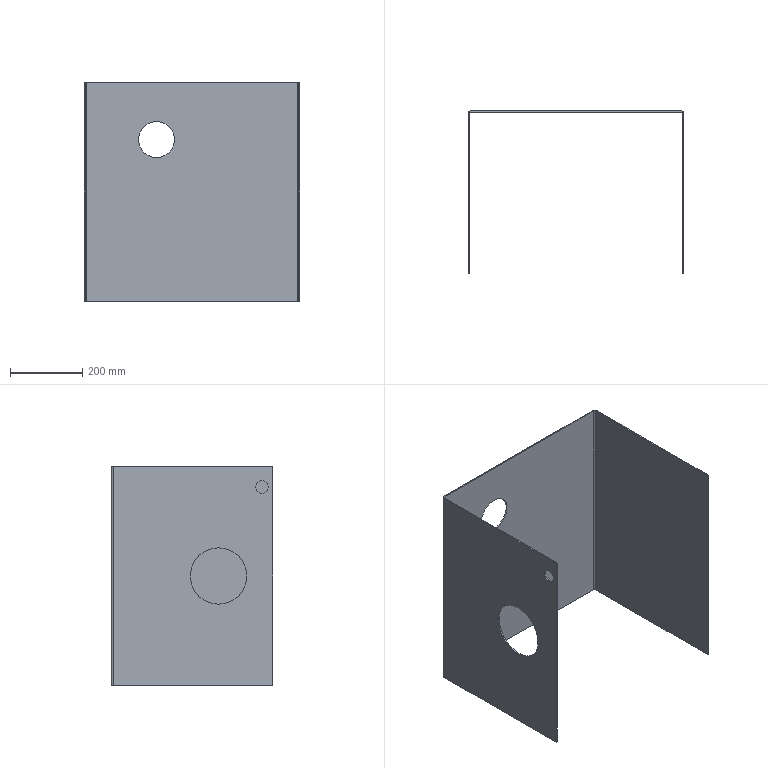Part | SolidWorks | features ICE 3, FlatPattern 1, SMBaseFlange 1, SheetMetal 1 | 1 solid | 32 faces | box 596 x 447 x 606 mm | volume 2607078 mm3 | plane 18 | cylinder 14 | commonest cylinder face diameters 6 x6 12 x2 35 x2 100 x2 156 x2
STEP:
#1=CARTESIAN_POINT('',(200.,447.,398.));
#2=VERTEX_POINT('',#1);
#3=CARTESIAN_POINT('',(200.,447.,498.));
#4=VERTEX_POINT('',#3);
#5=CARTESIAN_POINT('',(200.,447.,448.));
#6=DIRECTION('',(0.,1.,0.));
#7=DIRECTION('',(0.,0.,1.));
#8=AXIS2_PLACEMENT_3D('',#5,#6,#7);
#9=CIRCLE('',#8,50.);
#10=EDGE_CURVE('',#2,#4,#9,.T.);
#11=ORIENTED_EDGE('',*,*,#10,.T.);
#12=CARTESIAN_POINT('',(200.,444.,498.));
#13=VERTEX_POINT('',#12);
#14=CARTESIAN_POINT('',(200.,454.,498.));
#15=DIRECTION('',(0.,-1.,0.));
#16=VECTOR('',#15,1000.);
#17=LINE('',#14,#16);
#18=EDGE_CURVE('',#4,#13,#17,.T.);
#19=ORIENTED_EDGE('',*,*,#18,.T.);
#20=CARTESIAN_POINT('',(200.,444.,398.));
#21=VERTEX_POINT('',#20);
#22=CARTESIAN_POINT('',(200.,444.,448.));
#23=DIRECTION('',(0.,-1.,0.));
#24=DIRECTION('',(0.,0.,-1.));
#25=AXIS2_PLACEMENT_3D('',#22,#23,#24);
#26=CIRCLE('',#25,50.);
#27=EDGE_CURVE('',#13,#21,#26,.T.);
#28=ORIENTED_EDGE('',*,*,#27,.T.);
#29=CARTESIAN_POINT('',(200.,454.,398.));
#30=DIRECTION('',(0.,-1.,0.));
#31=VECTOR('',#30,1000.);
#32=LINE('',#29,#31);
#33=EDGE_CURVE('',#2,#21,#32,.T.);
#34=ORIENTED_EDGE('',*,*,#33,.F.);
#35=EDGE_LOOP('',(#11,#19,#28,#34));
#36=FACE_OUTER_BOUND('',#35,.T.);
#37=CARTESIAN_POINT('',(200.,454.,448.));
#38=DIRECTION('',(0.,-1.,0.));
#39=DIRECTION('',(0.,0.,-1.));
#40=AXIS2_PLACEMENT_3D('',#37,#38,#39);
#41=CYLINDRICAL_SURFACE('',#40,50.);
#42=ADVANCED_FACE('',(#36),#41,.F.);
#43=CARTESIAN_POINT('',(3.,30.,531.5));
#44=VERTEX_POINT('',#43);
#45=CARTESIAN_POINT('',(3.,30.,566.5));
#46=VERTEX_POINT('',#45);
#47=CARTESIAN_POINT('',(3.,30.,549.));
#48=DIRECTION('',(-1.,0.,0.));
#49=DIRECTION('',(0.,0.,1.));
#50=AXIS2_PLACEMENT_3D('',#47,#48,#49);
#51=CIRCLE('',#50,17.5);
#52=EDGE_CURVE('',#44,#46,#51,.T.);
#53=ORIENTED_EDGE('',*,*,#52,.F.);
#54=CARTESIAN_POINT('',(0.,30.,531.5));
#55=VERTEX_POINT('',#54);
#56=CARTESIAN_POINT('',(10.,30.,531.5));
#57=DIRECTION('',(-1.,0.,0.));
#58=VECTOR('',#57,1000.);
#59=LINE('',#56,#58);
#60=EDGE_CURVE('',#44,#55,#59,.T.);
#61=ORIENTED_EDGE('',*,*,#60,.T.);
#62=CARTESIAN_POINT('',(0.,30.,566.5));
#63=VERTEX_POINT('',#62);
#64=CARTESIAN_POINT('',(0.,30.,549.));
#65=DIRECTION('',(-1.,0.,0.));
#66=DIRECTION('',(0.,0.,1.));
#67=AXIS2_PLACEMENT_3D('',#64,#65,#66);
#68=CIRCLE('',#67,17.5);
#69=EDGE_CURVE('',#55,#63,#68,.T.);
#70=ORIENTED_EDGE('',*,*,#69,.T.);
#71=CARTESIAN_POINT('',(10.,30.,566.5));
#72=DIRECTION('',(-1.,0.,0.));
#73=VECTOR('',#72,1000.);
#74=LINE('',#71,#73);
#75=EDGE_CURVE('',#46,#63,#74,.T.);
#76=ORIENTED_EDGE('',*,*,#75,.F.);
#77=EDGE_LOOP('',(#53,#61,#70,#76));
#78=FACE_OUTER_BOUND('',#77,.T.);
#79=CARTESIAN_POINT('',(10.,30.,549.));
#80=DIRECTION('',(-1.,0.,0.));
#81=DIRECTION('',(0.,0.,1.));
#82=AXIS2_PLACEMENT_3D('',#79,#80,#81);
#83=CYLINDRICAL_SURFACE('',#82,17.5);
#84=ADVANCED_FACE('',(#78),#83,.F.);
#85=CARTESIAN_POINT('',(3.,150.,225.));
#86=VERTEX_POINT('',#85);
#87=CARTESIAN_POINT('',(3.,150.,381.));
#88=VERTEX_POINT('',#87);
#89=CARTESIAN_POINT('',(3.,150.,303.));
#90=DIRECTION('',(-1.,0.,0.));
#91=DIRECTION('',(0.,0.,1.));
#92=AXIS2_PLACEMENT_3D('',#89,#90,#91);
#93=CIRCLE('',#92,78.);
#94=EDGE_CURVE('',#86,#88,#93,.T.);
#95=ORIENTED_EDGE('',*,*,#94,.F.);
#96=CARTESIAN_POINT('',(0.,150.,225.));
#97=VERTEX_POINT('',#96);
#98=CARTESIAN_POINT('',(10.,150.,225.));
#99=DIRECTION('',(-1.,0.,0.));
#100=VECTOR('',#99,1000.);
#101=LINE('',#98,#100);
#102=EDGE_CURVE('',#86,#97,#101,.T.);
#103=ORIENTED_EDGE('',*,*,#102,.T.);
#104=CARTESIAN_POINT('',(0.,150.,381.));
#105=VERTEX_POINT('',#104);
#106=CARTESIAN_POINT('',(0.,150.,303.));
#107=DIRECTION('',(-1.,0.,0.));
#108=DIRECTION('',(0.,0.,1.));
#109=AXIS2_PLACEMENT_3D('',#106,#107,#108);
#110=CIRCLE('',#109,78.);
#111=EDGE_CURVE('',#97,#105,#110,.T.);
#112=ORIENTED_EDGE('',*,*,#111,.T.);
#113=CARTESIAN_POINT('',(10.,150.,381.));
#114=DIRECTION('',(-1.,0.,0.));
#115=VECTOR('',#114,1000.);
#116=LINE('',#113,#115);
#117=EDGE_CURVE('',#88,#105,#116,.T.);
#118=ORIENTED_EDGE('',*,*,#117,.F.);
#119=EDGE_LOOP('',(#95,#103,#112,#118));
#120=FACE_OUTER_BOUND('',#119,.T.);
#121=CARTESIAN_POINT('',(10.,150.,303.));
#122=DIRECTION('',(-1.,0.,0.));
#123=DIRECTION('',(0.,0.,1.));
#124=AXIS2_PLACEMENT_3D('',#121,#122,#123);
#125=CYLINDRICAL_SURFACE('',#124,78.);
#126=ADVANCED_FACE('',(#120),#125,.F.);
#127=CARTESIAN_POINT('',(593.,3.,606.));
#128=VERTEX_POINT('',#127);
#129=CARTESIAN_POINT('',(593.,0.,603.));
#130=VERTEX_POINT('',#129);
#131=CARTESIAN_POINT('',(593.,3.,603.));
#132=DIRECTION('',(1.,0.,0.));
#133=DIRECTION('',(0.,1.,0.));
#134=AXIS2_PLACEMENT_3D('',#131,#132,#133);
#135=CIRCLE('',#134,3.);
#136=EDGE_CURVE('',#128,#130,#135,.T.);
#137=ORIENTED_EDGE('',*,*,#136,.F.);
#138=CARTESIAN_POINT('',(593.,441.,606.));
#139=VERTEX_POINT('',#138);
#140=CARTESIAN_POINT('',(593.,447.,606.));
#141=DIRECTION('',(0.,-1.,0.));
#142=VECTOR('',#141,1000.);
#143=LINE('',#140,#142);
#144=EDGE_CURVE('',#139,#128,#143,.T.);
#145=ORIENTED_EDGE('',*,*,#144,.F.);
#146=CARTESIAN_POINT('',(593.,441.,0.));
#147=VERTEX_POINT('',#146);
#148=CARTESIAN_POINT('',(593.,441.,606.));
#149=DIRECTION('',(0.,0.,-1.));
#150=VECTOR('',#149,1000.);
#151=LINE('',#148,#150);
#152=EDGE_CURVE('',#139,#147,#151,.T.);
#153=ORIENTED_EDGE('',*,*,#152,.T.);
#154=CARTESIAN_POINT('',(593.,3.,0.));
#155=VERTEX_POINT('',#154);
#156=CARTESIAN_POINT('',(593.,447.,0.));
#157=DIRECTION('',(0.,-1.,0.));
#158=VECTOR('',#157,1000.);
#159=LINE('',#156,#158);
#160=EDGE_CURVE('',#147,#155,#159,.T.);
#161=ORIENTED_EDGE('',*,*,#160,.T.);
#162=CARTESIAN_POINT('',(593.,0.,3.));
#163=VERTEX_POINT('',#162);
#164=CARTESIAN_POINT('',(593.,3.,3.));
#165=DIRECTION('',(-1.,0.,0.));
#166=DIRECTION('',(0.,1.,0.));
#167=AXIS2_PLACEMENT_3D('',#164,#165,#166);
#168=CIRCLE('',#167,3.);
#169=EDGE_CURVE('',#155,#163,#168,.T.);
#170=ORIENTED_EDGE('',*,*,#169,.T.);
#171=CARTESIAN_POINT('',(593.,0.,606.));
#172=DIRECTION('',(0.,0.,-1.));
#173=VECTOR('',#172,1000.);
#174=LINE('',#171,#173);
#175=EDGE_CURVE('',#130,#163,#174,.T.);
#176=ORIENTED_EDGE('',*,*,#175,.F.);
#177=EDGE_LOOP('',(#137,#145,#153,#161,#170,#176));
#178=FACE_OUTER_BOUND('',#177,.T.);
#179=CARTESIAN_POINT('',(593.,447.,606.));
#180=DIRECTION('',(1.,0.,0.));
#181=DIRECTION('',(0.,1.,0.));
#182=AXIS2_PLACEMENT_3D('',#179,#180,#181);
#183=PLANE('',#182);
#184=ADVANCED_FACE('',(#178),#183,.F.);
#185=CARTESIAN_POINT('',(596.,441.,606.));
#186=VERTEX_POINT('',#185);
#187=CARTESIAN_POINT('',(596.,3.,606.));
#188=VERTEX_POINT('',#187);
#189=CARTESIAN_POINT('',(596.,447.,606.));
#190=DIRECTION('',(0.,-1.,0.));
#191=VECTOR('',#190,1000.);
#192=LINE('',#189,#191);
#193=EDGE_CURVE('',#186,#188,#192,.T.);
#194=ORIENTED_EDGE('',*,*,#193,.T.);
#195=CARTESIAN_POINT('',(596.,0.,603.));
#196=VERTEX_POINT('',#195);
#197=CARTESIAN_POINT('',(596.,3.,603.));
#198=DIRECTION('',(1.,0.,0.));
#199=DIRECTION('',(0.,1.,0.));
#200=AXIS2_PLACEMENT_3D('',#197,#198,#199);
#201=CIRCLE('',#200,3.);
#202=EDGE_CURVE('',#188,#196,#201,.T.);
#203=ORIENTED_EDGE('',*,*,#202,.T.);
#204=CARTESIAN_POINT('',(596.,0.,3.));
#205=VERTEX_POINT('',#204);
#206=CARTESIAN_POINT('',(596.,0.,606.));
#207=DIRECTION('',(0.,0.,-1.));
#208=VECTOR('',#207,1000.);
#209=LINE('',#206,#208);
#210=EDGE_CURVE('',#196,#205,#209,.T.);
#211=ORIENTED_EDGE('',*,*,#210,.T.);
#212=CARTESIAN_POINT('',(596.,3.,0.));
#213=VERTEX_POINT('',#212);
#214=CARTESIAN_POINT('',(596.,3.,3.));
#215=DIRECTION('',(-1.,0.,0.));
#216=DIRECTION('',(0.,1.,0.));
#217=AXIS2_PLACEMENT_3D('',#214,#215,#216);
#218=CIRCLE('',#217,3.);
#219=EDGE_CURVE('',#213,#205,#218,.T.);
#220=ORIENTED_EDGE('',*,*,#219,.F.);
#221=CARTESIAN_POINT('',(596.,441.,0.));
#222=VERTEX_POINT('',#221);
#223=CARTESIAN_POINT('',(596.,447.,0.));
#224=DIRECTION('',(0.,-1.,0.));
#225=VECTOR('',#224,1000.);
#226=LINE('',#223,#225);
#227=EDGE_CURVE('',#222,#213,#226,.T.);
#228=ORIENTED_EDGE('',*,*,#227,.F.);
#229=CARTESIAN_POINT('',(596.,441.,606.));
#230=DIRECTION('',(0.,0.,-1.));
#231=VECTOR('',#230,1000.);
#232=LINE('',#229,#231);
#233=EDGE_CURVE('',#186,#222,#232,.T.);
#234=ORIENTED_EDGE('',*,*,#233,.F.);
#235=EDGE_LOOP('',(#194,#203,#211,#220,#228,#234));
#236=FACE_OUTER_BOUND('',#235,.T.);
#237=CARTESIAN_POINT('',(596.,447.,606.));
#238=DIRECTION('',(1.,0.,0.));
#239=DIRECTION('',(0.,1.,0.));
#240=AXIS2_PLACEMENT_3D('',#237,#238,#239);
#241=PLANE('',#240);
#242=ADVANCED_FACE('',(#236),#241,.T.);
#243=ORIENTED_EDGE('',*,*,#144,.T.);
#244=CARTESIAN_POINT('',(593.,3.,606.));
#245=DIRECTION('',(1.,0.,0.));
#246=VECTOR('',#245,1000.);
#247=LINE('',#244,#246);
#248=EDGE_CURVE('',#128,#188,#247,.T.);
#249=ORIENTED_EDGE('',*,*,#248,.T.);
#250=ORIENTED_EDGE('',*,*,#193,.F.);
#251=CARTESIAN_POINT('',(596.,441.,606.));
#252=DIRECTION('',(-1.,0.,0.));
#253=VECTOR('',#252,1000.);
#254=LINE('',#251,#253);
#255=EDGE_CURVE('',#186,#139,#254,.T.);
#256=ORIENTED_EDGE('',*,*,#255,.T.);
#257=EDGE_LOOP('',(#243,#249,#250,#256));
#258=FACE_OUTER_BOUND('',#257,.T.);
#259=CARTESIAN_POINT('',(590.,444.,606.));
#260=DIRECTION('',(0.,0.,1.));
#261=DIRECTION('',(1.,0.,0.));
#262=AXIS2_PLACEMENT_3D('',#259,#260,#261);
#263=PLANE('',#262);
#264=ADVANCED_FACE('',(#258),#263,.T.);
#265=CARTESIAN_POINT('',(593.,0.,603.));
#266=DIRECTION('',(1.,0.,0.));
#267=VECTOR('',#266,1000.);
#268=LINE('',#265,#267);
#269=EDGE_CURVE('',#130,#196,#268,.T.);
#270=ORIENTED_EDGE('',*,*,#269,.F.);
#271=ORIENTED_EDGE('',*,*,#175,.T.);
#272=CARTESIAN_POINT('',(593.,0.,3.));
#273=DIRECTION('',(1.,0.,0.));
#274=VECTOR('',#273,1000.);
#275=LINE('',#272,#274);
#276=EDGE_CURVE('',#163,#205,#275,.T.);
#277=ORIENTED_EDGE('',*,*,#276,.T.);
#278=ORIENTED_EDGE('',*,*,#210,.F.);
#279=EDGE_LOOP('',(#270,#271,#277,#278));
#280=FACE_OUTER_BOUND('',#279,.T.);
#281=CARTESIAN_POINT('',(596.,0.,606.));
#282=DIRECTION('',(0.,-1.,0.));
#283=DIRECTION('',(0.,0.,-1.));
#284=AXIS2_PLACEMENT_3D('',#281,#282,#283);
#285=PLANE('',#284);
#286=ADVANCED_FACE('',(#280),#285,.T.);
#287=CARTESIAN_POINT('',(593.,3.,0.));
#288=DIRECTION('',(1.,0.,0.));
#289=VECTOR('',#288,1000.);
#290=LINE('',#287,#289);
#291=EDGE_CURVE('',#155,#213,#290,.T.);
#292=ORIENTED_EDGE('',*,*,#291,.F.);
#293=ORIENTED_EDGE('',*,*,#160,.F.);
#294=CARTESIAN_POINT('',(593.,441.,0.));
#295=DIRECTION('',(1.,0.,0.));
#296=VECTOR('',#295,1000.);
#297=LINE('',#294,#296);
#298=EDGE_CURVE('',#147,#222,#297,.T.);
#299=ORIENTED_EDGE('',*,*,#298,.T.);
#300=ORIENTED_EDGE('',*,*,#227,.T.);
#301=EDGE_LOOP('',(#292,#293,#299,#300));
#302=FACE_OUTER_BOUND('',#301,.T.);
#303=CARTESIAN_POINT('',(590.,441.,0.));
#304=DIRECTION('',(0.,0.,1.));
#305=DIRECTION('',(1.,0.,0.));
#306=AXIS2_PLACEMENT_3D('',#303,#304,#305);
#307=PLANE('',#306);
#308=ADVANCED_FACE('',(#302),#307,.F.);
#309=CARTESIAN_POINT('',(0.,30.,549.));
#310=DIRECTION('',(-1.,0.,0.));
#311=DIRECTION('',(0.,0.,1.));
#312=AXIS2_PLACEMENT_3D('',#309,#310,#311);
#313=CIRCLE('',#312,17.5);
#314=EDGE_CURVE('',#63,#55,#313,.T.);
#315=ORIENTED_EDGE('',*,*,#314,.F.);
#316=ORIENTED_EDGE('',*,*,#69,.F.);
#317=EDGE_LOOP('',(#315,#316));
#318=FACE_BOUND('',#317,.T.);
#319=CARTESIAN_POINT('',(0.,150.,303.));
#320=DIRECTION('',(-1.,0.,0.));
#321=DIRECTION('',(0.,0.,1.));
#322=AXIS2_PLACEMENT_3D('',#319,#320,#321);
#323=CIRCLE('',#322,78.);
#324=EDGE_CURVE('',#105,#97,#323,.T.);
#325=ORIENTED_EDGE('',*,*,#324,.F.);
#326=ORIENTED_EDGE('',*,*,#111,.F.);
#327=EDGE_LOOP('',(#325,#326));
#328=FACE_BOUND('',#327,.T.);
#329=CARTESIAN_POINT('',(0.,0.,603.));
#330=VERTEX_POINT('',#329);
#331=CARTESIAN_POINT('',(0.,0.,3.));
#332=VERTEX_POINT('',#331);
#333=CARTESIAN_POINT('',(0.,0.,606.));
#334=DIRECTION('',(0.,0.,-1.));
#335=VECTOR('',#334,1000.);
#336=LINE('',#333,#335);
#337=EDGE_CURVE('',#330,#332,#336,.T.);
#338=ORIENTED_EDGE('',*,*,#337,.F.);
#339=CARTESIAN_POINT('',(0.,3.,606.));
#340=VERTEX_POINT('',#339);
#341=CARTESIAN_POINT('',(0.,3.,603.));
#342=DIRECTION('',(-1.,0.,0.));
#343=DIRECTION('',(0.,0.,1.));
#344=AXIS2_PLACEMENT_3D('',#341,#342,#343);
#345=CIRCLE('',#344,3.);
#346=EDGE_CURVE('',#330,#340,#345,.T.);
#347=ORIENTED_EDGE('',*,*,#346,.T.);
#348=CARTESIAN_POINT('',(0.,441.,606.));
#349=VERTEX_POINT('',#348);
#350=CARTESIAN_POINT('',(0.,0.,606.));
#351=DIRECTION('',(0.,1.,0.));
#352=VECTOR('',#351,1000.);
#353=LINE('',#350,#352);
#354=EDGE_CURVE('',#340,#349,#353,.T.);
#355=ORIENTED_EDGE('',*,*,#354,.T.);
#356=CARTESIAN_POINT('',(0.,441.,0.));
#357=VERTEX_POINT('',#356);
#358=CARTESIAN_POINT('',(0.,441.,606.));
#359=DIRECTION('',(0.,0.,-1.));
#360=VECTOR('',#359,1000.);
#361=LINE('',#358,#360);
#362=EDGE_CURVE('',#349,#357,#361,.T.);
#363=ORIENTED_EDGE('',*,*,#362,.T.);
#364=CARTESIAN_POINT('',(0.,3.,0.));
#365=VERTEX_POINT('',#364);
#366=CARTESIAN_POINT('',(0.,0.,0.));
#367=DIRECTION('',(0.,1.,0.));
#368=VECTOR('',#367,1000.);
#369=LINE('',#366,#368);
#370=EDGE_CURVE('',#365,#357,#369,.T.);
#371=ORIENTED_EDGE('',*,*,#370,.F.);
#372=CARTESIAN_POINT('',(0.,3.,3.));
#373=DIRECTION('',(1.,0.,0.));
#374=DIRECTION('',(0.,0.,1.));
#375=AXIS2_PLACEMENT_3D('',#372,#373,#374);
#376=CIRCLE('',#375,3.);
#377=EDGE_CURVE('',#332,#365,#376,.T.);
#378=ORIENTED_EDGE('',*,*,#377,.F.);
#379=EDGE_LOOP('',(#338,#347,#355,#363,#371,#378));
#380=FACE_OUTER_BOUND('',#379,.T.);
#381=CARTESIAN_POINT('',(0.,0.,606.));
#382=DIRECTION('',(-1.,0.,0.));
#383=DIRECTION('',(0.,0.,1.));
#384=AXIS2_PLACEMENT_3D('',#381,#382,#383);
#385=PLANE('',#384);
#386=ADVANCED_FACE('',(#318,#328,#380),#385,.T.);
#387=CARTESIAN_POINT('',(3.,30.,549.));
#388=DIRECTION('',(-1.,0.,0.));
#389=DIRECTION('',(0.,0.,1.));
#390=AXIS2_PLACEMENT_3D('',#387,#388,#389);
#391=CIRCLE('',#390,17.5);
#392=EDGE_CURVE('',#46,#44,#391,.T.);
#393=ORIENTED_EDGE('',*,*,#392,.T.);
#394=ORIENTED_EDGE('',*,*,#52,.T.);
#395=EDGE_LOOP('',(#393,#394));
#396=FACE_BOUND('',#395,.T.);
#397=CARTESIAN_POINT('',(3.,150.,303.));
#398=DIRECTION('',(-1.,0.,0.));
#399=DIRECTION('',(0.,0.,1.));
#400=AXIS2_PLACEMENT_3D('',#397,#398,#399);
#401=CIRCLE('',#400,78.);
#402=EDGE_CURVE('',#88,#86,#401,.T.);
#403=ORIENTED_EDGE('',*,*,#402,.T.);
#404=ORIENTED_EDGE('',*,*,#94,.T.);
#405=EDGE_LOOP('',(#403,#404));
#406=FACE_BOUND('',#405,.T.);
#407=CARTESIAN_POINT('',(3.,0.,603.));
#408=VERTEX_POINT('',#407);
#409=CARTESIAN_POINT('',(3.,3.,606.));
#410=VERTEX_POINT('',#409);
#411=CARTESIAN_POINT('',(3.,3.,603.));
#412=DIRECTION('',(-1.,0.,0.));
#413=DIRECTION('',(0.,0.,1.));
#414=AXIS2_PLACEMENT_3D('',#411,#412,#413);
#415=CIRCLE('',#414,3.);
#416=EDGE_CURVE('',#408,#410,#415,.T.);
#417=ORIENTED_EDGE('',*,*,#416,.F.);
#418=CARTESIAN_POINT('',(3.,0.,3.));
#419=VERTEX_POINT('',#418);
#420=CARTESIAN_POINT('',(3.,0.,606.));
#421=DIRECTION('',(0.,0.,-1.));
#422=VECTOR('',#421,1000.);
#423=LINE('',#420,#422);
#424=EDGE_CURVE('',#408,#419,#423,.T.);
#425=ORIENTED_EDGE('',*,*,#424,.T.);
#426=CARTESIAN_POINT('',(3.,3.,0.));
#427=VERTEX_POINT('',#426);
#428=CARTESIAN_POINT('',(3.,3.,3.));
#429=DIRECTION('',(1.,0.,0.));
#430=DIRECTION('',(0.,0.,1.));
#431=AXIS2_PLACEMENT_3D('',#428,#429,#430);
#432=CIRCLE('',#431,3.);
#433=EDGE_CURVE('',#419,#427,#432,.T.);
#434=ORIENTED_EDGE('',*,*,#433,.T.);
#435=CARTESIAN_POINT('',(3.,441.,0.));
#436=VERTEX_POINT('',#435);
#437=CARTESIAN_POINT('',(3.,0.,0.));
#438=DIRECTION('',(0.,1.,0.));
#439=VECTOR('',#438,1000.);
#440=LINE('',#437,#439);
#441=EDGE_CURVE('',#427,#436,#440,.T.);
#442=ORIENTED_EDGE('',*,*,#441,.T.);
#443=CARTESIAN_POINT('',(3.,441.,606.));
#444=VERTEX_POINT('',#443);
#445=CARTESIAN_POINT('',(3.,441.,606.));
#446=DIRECTION('',(0.,0.,-1.));
#447=VECTOR('',#446,1000.);
#448=LINE('',#445,#447);
#449=EDGE_CURVE('',#444,#436,#448,.T.);
#450=ORIENTED_EDGE('',*,*,#449,.F.);
#451=CARTESIAN_POINT('',(3.,0.,606.));
#452=DIRECTION('',(0.,1.,0.));
#453=VECTOR('',#452,1000.);
#454=LINE('',#451,#453);
#455=EDGE_CURVE('',#410,#444,#454,.T.);
#456=ORIENTED_EDGE('',*,*,#455,.F.);
#457=EDGE_LOOP('',(#417,#425,#434,#442,#450,#456));
#458=FACE_OUTER_BOUND('',#457,.T.);
#459=CARTESIAN_POINT('',(3.,0.,606.));
#460=DIRECTION('',(-1.,0.,0.));
#461=DIRECTION('',(0.,0.,1.));
#462=AXIS2_PLACEMENT_3D('',#459,#460,#461);
#463=PLANE('',#462);
#464=ADVANCED_FACE('',(#396,#406,#458),#463,.F.);
#465=ORIENTED_EDGE('',*,*,#424,.F.);
#466=CARTESIAN_POINT('',(3.,0.,603.));
#467=DIRECTION('',(-1.,0.,0.));
#468=VECTOR('',#467,1000.);
#469=LINE('',#466,#468);
#470=EDGE_CURVE('',#408,#330,#469,.T.);
#471=ORIENTED_EDGE('',*,*,#470,.T.);
#472=ORIENTED_EDGE('',*,*,#337,.T.);
#473=CARTESIAN_POINT('',(3.,0.,3.));
#474=DIRECTION('',(-1.,0.,0.));
#475=VECTOR('',#474,1000.);
#476=LINE('',#473,#475);
#477=EDGE_CURVE('',#419,#332,#476,.T.);
#478=ORIENTED_EDGE('',*,*,#477,.F.);
#479=EDGE_LOOP('',(#465,#471,#472,#478));
#480=FACE_OUTER_BOUND('',#479,.T.);
#481=CARTESIAN_POINT('',(3.,0.,606.));
#482=DIRECTION('',(0.,-1.,0.));
#483=DIRECTION('',(0.,0.,-1.));
#484=AXIS2_PLACEMENT_3D('',#481,#482,#483);
#485=PLANE('',#484);
#486=ADVANCED_FACE('',(#480),#485,.T.);
#487=ORIENTED_EDGE('',*,*,#441,.F.);
#488=CARTESIAN_POINT('',(3.,3.,0.));
#489=DIRECTION('',(-1.,0.,0.));
#490=VECTOR('',#489,1000.);
#491=LINE('',#488,#490);
#492=EDGE_CURVE('',#427,#365,#491,.T.);
#493=ORIENTED_EDGE('',*,*,#492,.T.);
#494=ORIENTED_EDGE('',*,*,#370,.T.);
#495=CARTESIAN_POINT('',(0.,441.,0.));
#496=DIRECTION('',(1.,0.,0.));
#497=VECTOR('',#496,1000.);
#498=LINE('',#495,#497);
#499=EDGE_CURVE('',#357,#436,#498,.T.);
#500=ORIENTED_EDGE('',*,*,#499,.T.);
#501=EDGE_LOOP('',(#487,#493,#494,#500));
#502=FACE_OUTER_BOUND('',#501,.T.);
#503=CARTESIAN_POINT('',(6.,444.,0.));
#504=DIRECTION('',(0.,0.,-1.));
#505=DIRECTION('',(-1.,0.,0.));
#506=AXIS2_PLACEMENT_3D('',#503,#504,#505);
#507=PLANE('',#506);
#508=ADVANCED_FACE('',(#502),#507,.T.);
#509=CARTESIAN_POINT('',(6.,447.,606.));
#510=VERTEX_POINT('',#509);
#511=CARTESIAN_POINT('',(6.,444.,606.));
#512=VERTEX_POINT('',#511);
#513=CARTESIAN_POINT('',(6.,447.,606.));
#514=DIRECTION('',(0.,-1.,0.));
#515=VECTOR('',#514,1000.);
#516=LINE('',#513,#515);
#517=EDGE_CURVE('',#510,#512,#516,.T.);
#518=ORIENTED_EDGE('',*,*,#517,.F.);
#519=CARTESIAN_POINT('',(6.,441.,606.));
#520=DIRECTION('',(0.,0.,-1.));
#521=DIRECTION('',(1.,0.,0.));
#522=AXIS2_PLACEMENT_3D('',#519,#520,#521);
#523=CIRCLE('',#522,6.);
#524=EDGE_CURVE('',#349,#510,#523,.T.);
#525=ORIENTED_EDGE('',*,*,#524,.F.);
#526=CARTESIAN_POINT('',(3.,441.,606.));
#527=DIRECTION('',(-1.,0.,0.));
#528=VECTOR('',#527,1000.);
#529=LINE('',#526,#528);
#530=EDGE_CURVE('',#444,#349,#529,.T.);
#531=ORIENTED_EDGE('',*,*,#530,.F.);
#532=CARTESIAN_POINT('',(6.,441.,606.));
#533=DIRECTION('',(0.,0.,-1.));
#534=DIRECTION('',(1.,0.,0.));
#535=AXIS2_PLACEMENT_3D('',#532,#533,#534);
#536=CIRCLE('',#535,3.);
#537=EDGE_CURVE('',#444,#512,#536,.T.);
#538=ORIENTED_EDGE('',*,*,#537,.T.);
#539=EDGE_LOOP('',(#518,#525,#531,#538));
#540=FACE_OUTER_BOUND('',#539,.T.);
#541=CARTESIAN_POINT('',(6.,447.,606.));
#542=DIRECTION('',(0.,0.,1.));
#543=DIRECTION('',(1.,0.,0.));
#544=AXIS2_PLACEMENT_3D('',#541,#542,#543);
#545=PLANE('',#544);
#546=ADVANCED_FACE('',(#540),#545,.T.);
#547=CARTESIAN_POINT('',(590.,447.,606.));
#548=VERTEX_POINT('',#547);
#549=CARTESIAN_POINT('',(0.,447.,606.));
#550=DIRECTION('',(1.,0.,0.));
#551=VECTOR('',#550,1000.);
#552=LINE('',#549,#551);
#553=EDGE_CURVE('',#510,#548,#552,.T.);
#554=ORIENTED_EDGE('',*,*,#553,.F.);
#555=ORIENTED_EDGE('',*,*,#517,.T.);
#556=CARTESIAN_POINT('',(590.,444.,606.));
#557=VERTEX_POINT('',#556);
#558=CARTESIAN_POINT('',(0.,444.,606.));
#559=DIRECTION('',(1.,0.,0.));
#560=VECTOR('',#559,1000.);
#561=LINE('',#558,#560);
#562=EDGE_CURVE('',#512,#557,#561,.T.);
#563=ORIENTED_EDGE('',*,*,#562,.T.);
#564=CARTESIAN_POINT('',(590.,444.,606.));
#565=DIRECTION('',(0.,1.,0.));
#566=VECTOR('',#565,1000.);
#567=LINE('',#564,#566);
#568=EDGE_CURVE('',#557,#548,#567,.T.);
#569=ORIENTED_EDGE('',*,*,#568,.T.);
#570=EDGE_LOOP('',(#554,#555,#563,#569));
#571=FACE_OUTER_BOUND('',#570,.T.);
#572=CARTESIAN_POINT('',(3.,441.,606.));
#573=DIRECTION('',(0.,0.,1.));
#574=DIRECTION('',(1.,0.,0.));
#575=AXIS2_PLACEMENT_3D('',#572,#573,#574);
#576=PLANE('',#575);
#577=ADVANCED_FACE('',(#571),#576,.T.);
#578=ORIENTED_EDGE('',*,*,#499,.F.);
#579=CARTESIAN_POINT('',(6.,447.,0.));
#580=VERTEX_POINT('',#579);
#581=CARTESIAN_POINT('',(6.,441.,0.));
#582=DIRECTION('',(0.,0.,-1.));
#583=DIRECTION('',(1.,0.,0.));
#584=AXIS2_PLACEMENT_3D('',#581,#582,#583);
#585=CIRCLE('',#584,6.);
#586=EDGE_CURVE('',#357,#580,#585,.T.);
#587=ORIENTED_EDGE('',*,*,#586,.T.);
#588=CARTESIAN_POINT('',(6.,444.,0.));
#589=VERTEX_POINT('',#588);
#590=CARTESIAN_POINT('',(6.,444.,0.));
#591=DIRECTION('',(0.,1.,0.));
#592=VECTOR('',#591,1000.);
#593=LINE('',#590,#592);
#594=EDGE_CURVE('',#589,#580,#593,.T.);
#595=ORIENTED_EDGE('',*,*,#594,.F.);
#596=CARTESIAN_POINT('',(6.,441.,0.));
#597=DIRECTION('',(0.,0.,-1.));
#598=DIRECTION('',(1.,0.,0.));
#599=AXIS2_PLACEMENT_3D('',#596,#597,#598);
#600=CIRCLE('',#599,3.);
#601=EDGE_CURVE('',#436,#589,#600,.T.);
#602=ORIENTED_EDGE('',*,*,#601,.F.);
#603=EDGE_LOOP('',(#578,#587,#595,#602));
#604=FACE_OUTER_BOUND('',#603,.T.);
#605=CARTESIAN_POINT('',(0.,441.,0.));
#606=DIRECTION('',(0.,0.,-1.));
#607=DIRECTION('',(-1.,0.,0.));
#608=AXIS2_PLACEMENT_3D('',#605,#606,#607);
#609=PLANE('',#608);
#610=ADVANCED_FACE('',(#604),#609,.T.);
#611=ORIENTED_EDGE('',*,*,#255,.F.);
#612=CARTESIAN_POINT('',(590.,441.,606.));
#613=DIRECTION('',(0.,0.,-1.));
#614=DIRECTION('',(1.,0.,0.));
#615=AXIS2_PLACEMENT_3D('',#612,#613,#614);
#616=CIRCLE('',#615,6.);
#617=EDGE_CURVE('',#548,#186,#616,.T.);
#618=ORIENTED_EDGE('',*,*,#617,.F.);
#619=ORIENTED_EDGE('',*,*,#568,.F.);
#620=CARTESIAN_POINT('',(590.,441.,606.));
#621=DIRECTION('',(0.,0.,-1.));
#622=DIRECTION('',(1.,0.,0.));
#623=AXIS2_PLACEMENT_3D('',#620,#621,#622);
#624=CIRCLE('',#623,3.);
#625=EDGE_CURVE('',#557,#139,#624,.T.);
#626=ORIENTED_EDGE('',*,*,#625,.T.);
#627=EDGE_LOOP('',(#611,#618,#619,#626));
#628=FACE_OUTER_BOUND('',#627,.T.);
#629=CARTESIAN_POINT('',(596.,441.,606.));
#630=DIRECTION('',(0.,0.,1.));
#631=DIRECTION('',(1.,0.,0.));
#632=AXIS2_PLACEMENT_3D('',#629,#630,#631);
#633=PLANE('',#632);
#634=ADVANCED_FACE('',(#628),#633,.T.);
#635=CARTESIAN_POINT('',(590.,447.,0.));
#636=VERTEX_POINT('',#635);
#637=CARTESIAN_POINT('',(590.,444.,0.));
#638=VERTEX_POINT('',#637);
#639=CARTESIAN_POINT('',(590.,447.,0.));
#640=DIRECTION('',(0.,-1.,0.));
#641=VECTOR('',#640,1000.);
#642=LINE('',#639,#641);
#643=EDGE_CURVE('',#636,#638,#642,.T.);
#644=ORIENTED_EDGE('',*,*,#643,.F.);
#645=CARTESIAN_POINT('',(590.,441.,0.));
#646=DIRECTION('',(0.,0.,-1.));
#647=DIRECTION('',(1.,0.,0.));
#648=AXIS2_PLACEMENT_3D('',#645,#646,#647);
#649=CIRCLE('',#648,6.);
#650=EDGE_CURVE('',#636,#222,#649,.T.);
#651=ORIENTED_EDGE('',*,*,#650,.T.);
#652=ORIENTED_EDGE('',*,*,#298,.F.);
#653=CARTESIAN_POINT('',(590.,441.,0.));
#654=DIRECTION('',(0.,0.,-1.));
#655=DIRECTION('',(1.,0.,0.));
#656=AXIS2_PLACEMENT_3D('',#653,#654,#655);
#657=CIRCLE('',#656,3.);
#658=EDGE_CURVE('',#638,#147,#657,.T.);
#659=ORIENTED_EDGE('',*,*,#658,.F.);
#660=EDGE_LOOP('',(#644,#651,#652,#659));
#661=FACE_OUTER_BOUND('',#660,.T.);
#662=CARTESIAN_POINT('',(590.,447.,0.));
#663=DIRECTION('',(0.,0.,-1.));
#664=DIRECTION('',(-1.,0.,0.));
#665=AXIS2_PLACEMENT_3D('',#662,#663,#664);
#666=PLANE('',#665);
#667=ADVANCED_FACE('',(#661),#666,.T.);
#668=CARTESIAN_POINT('',(0.,447.,0.));
#669=DIRECTION('',(1.,0.,0.));
#670=VECTOR('',#669,1000.);
#671=LINE('',#668,#670);
#672=EDGE_CURVE('',#580,#636,#671,.T.);
#673=ORIENTED_EDGE('',*,*,#672,.T.);
#674=ORIENTED_EDGE('',*,*,#643,.T.);
#675=CARTESIAN_POINT('',(0.,444.,0.));
#676=DIRECTION('',(1.,0.,0.));
#677=VECTOR('',#676,1000.);
#678=LINE('',#675,#677);
#679=EDGE_CURVE('',#589,#638,#678,.T.);
#680=ORIENTED_EDGE('',*,*,#679,.F.);
#681=ORIENTED_EDGE('',*,*,#594,.T.);
#682=EDGE_LOOP('',(#673,#674,#680,#681));
#683=FACE_OUTER_BOUND('',#682,.T.);
#684=CARTESIAN_POINT('',(593.,441.,0.));
#685=DIRECTION('',(0.,0.,-1.));
#686=DIRECTION('',(-1.,0.,0.));
#687=AXIS2_PLACEMENT_3D('',#684,#685,#686);
#688=PLANE('',#687);
#689=ADVANCED_FACE('',(#683),#688,.T.);
#690=ORIENTED_EDGE('',*,*,#650,.F.);
#691=CARTESIAN_POINT('',(590.,447.,606.));
#692=DIRECTION('',(0.,0.,-1.));
#693=VECTOR('',#692,1000.);
#694=LINE('',#691,#693);
#695=EDGE_CURVE('',#548,#636,#694,.T.);
#696=ORIENTED_EDGE('',*,*,#695,.F.);
#697=ORIENTED_EDGE('',*,*,#617,.T.);
#698=ORIENTED_EDGE('',*,*,#233,.T.);
#699=EDGE_LOOP('',(#690,#696,#697,#698));
#700=FACE_OUTER_BOUND('',#699,.T.);
#701=CARTESIAN_POINT('',(590.,441.,606.));
#702=DIRECTION('',(0.,0.,-1.));
#703=DIRECTION('',(-1.,0.,0.));
#704=AXIS2_PLACEMENT_3D('',#701,#702,#703);
#705=CYLINDRICAL_SURFACE('',#704,6.);
#706=ADVANCED_FACE('',(#700),#705,.T.);
#707=ORIENTED_EDGE('',*,*,#10,.F.);
#708=CARTESIAN_POINT('',(200.,447.,448.));
#709=DIRECTION('',(0.,1.,0.));
#710=DIRECTION('',(0.,0.,1.));
#711=AXIS2_PLACEMENT_3D('',#708,#709,#710);
#712=CIRCLE('',#711,50.);
#713=EDGE_CURVE('',#4,#2,#712,.T.);
#714=ORIENTED_EDGE('',*,*,#713,.F.);
#715=EDGE_LOOP('',(#707,#714));
#716=FACE_BOUND('',#715,.T.);
#717=ORIENTED_EDGE('',*,*,#672,.F.);
#718=CARTESIAN_POINT('',(6.,447.,606.));
#719=DIRECTION('',(0.,0.,-1.));
#720=VECTOR('',#719,1000.);
#721=LINE('',#718,#720);
#722=EDGE_CURVE('',#510,#580,#721,.T.);
#723=ORIENTED_EDGE('',*,*,#722,.F.);
#724=ORIENTED_EDGE('',*,*,#553,.T.);
#725=ORIENTED_EDGE('',*,*,#695,.T.);
#726=EDGE_LOOP('',(#717,#723,#724,#725));
#727=FACE_OUTER_BOUND('',#726,.T.);
#728=CARTESIAN_POINT('',(0.,447.,606.));
#729=DIRECTION('',(0.,1.,0.));
#730=DIRECTION('',(0.,0.,1.));
#731=AXIS2_PLACEMENT_3D('',#728,#729,#730);
#732=PLANE('',#731);
#733=ADVANCED_FACE('',(#716,#727),#732,.T.);
#734=ORIENTED_EDGE('',*,*,#586,.F.);
#735=ORIENTED_EDGE('',*,*,#362,.F.);
#736=ORIENTED_EDGE('',*,*,#524,.T.);
#737=ORIENTED_EDGE('',*,*,#722,.T.);
#738=EDGE_LOOP('',(#734,#735,#736,#737));
#739=FACE_OUTER_BOUND('',#738,.T.);
#740=CARTESIAN_POINT('',(6.,441.,606.));
#741=DIRECTION('',(0.,0.,-1.));
#742=DIRECTION('',(-1.,0.,0.));
#743=AXIS2_PLACEMENT_3D('',#740,#741,#742);
#744=CYLINDRICAL_SURFACE('',#743,6.);
#745=ADVANCED_FACE('',(#739),#744,.T.);
#746=ORIENTED_EDGE('',*,*,#601,.T.);
#747=CARTESIAN_POINT('',(6.,444.,606.));
#748=DIRECTION('',(0.,0.,-1.));
#749=VECTOR('',#748,1000.);
#750=LINE('',#747,#749);
#751=EDGE_CURVE('',#512,#589,#750,.T.);
#752=ORIENTED_EDGE('',*,*,#751,.F.);
#753=ORIENTED_EDGE('',*,*,#537,.F.);
#754=ORIENTED_EDGE('',*,*,#449,.T.);
#755=EDGE_LOOP('',(#746,#752,#753,#754));
#756=FACE_OUTER_BOUND('',#755,.T.);
#757=CARTESIAN_POINT('',(6.,441.,606.));
#758=DIRECTION('',(0.,0.,-1.));
#759=DIRECTION('',(-1.,0.,0.));
#760=AXIS2_PLACEMENT_3D('',#757,#758,#759);
#761=CYLINDRICAL_SURFACE('',#760,3.);
#762=ADVANCED_FACE('',(#756),#761,.F.);
#763=CARTESIAN_POINT('',(200.,444.,448.));
#764=DIRECTION('',(0.,-1.,0.));
#765=DIRECTION('',(0.,0.,-1.));
#766=AXIS2_PLACEMENT_3D('',#763,#764,#765);
#767=CIRCLE('',#766,50.);
#768=EDGE_CURVE('',#21,#13,#767,.T.);
#769=ORIENTED_EDGE('',*,*,#768,.F.);
#770=ORIENTED_EDGE('',*,*,#27,.F.);
#771=EDGE_LOOP('',(#769,#770));
#772=FACE_BOUND('',#771,.T.);
#773=ORIENTED_EDGE('',*,*,#679,.T.);
#774=CARTESIAN_POINT('',(590.,444.,606.));
#775=DIRECTION('',(0.,0.,-1.));
#776=VECTOR('',#775,1000.);
#777=LINE('',#774,#776);
#778=EDGE_CURVE('',#557,#638,#777,.T.);
#779=ORIENTED_EDGE('',*,*,#778,.F.);
#780=ORIENTED_EDGE('',*,*,#562,.F.);
#781=ORIENTED_EDGE('',*,*,#751,.T.);
#782=EDGE_LOOP('',(#773,#779,#780,#781));
#783=FACE_OUTER_BOUND('',#782,.T.);
#784=CARTESIAN_POINT('',(0.,444.,606.));
#785=DIRECTION('',(0.,1.,0.));
#786=DIRECTION('',(0.,0.,1.));
#787=AXIS2_PLACEMENT_3D('',#784,#785,#786);
#788=PLANE('',#787);
#789=ADVANCED_FACE('',(#772,#783),#788,.F.);
#790=ORIENTED_EDGE('',*,*,#658,.T.);
#791=ORIENTED_EDGE('',*,*,#152,.F.);
#792=ORIENTED_EDGE('',*,*,#625,.F.);
#793=ORIENTED_EDGE('',*,*,#778,.T.);
#794=EDGE_LOOP('',(#790,#791,#792,#793));
#795=FACE_OUTER_BOUND('',#794,.T.);
#796=CARTESIAN_POINT('',(590.,441.,606.));
#797=DIRECTION('',(0.,0.,-1.));
#798=DIRECTION('',(-1.,0.,0.));
#799=AXIS2_PLACEMENT_3D('',#796,#797,#798);
#800=CYLINDRICAL_SURFACE('',#799,3.);
#801=ADVANCED_FACE('',(#795),#800,.F.);
#802=CARTESIAN_POINT('',(3.,3.,606.));
#803=DIRECTION('',(-1.,0.,0.));
#804=VECTOR('',#803,1000.);
#805=LINE('',#802,#804);
#806=EDGE_CURVE('',#410,#340,#805,.T.);
#807=ORIENTED_EDGE('',*,*,#806,.F.);
#808=ORIENTED_EDGE('',*,*,#455,.T.);
#809=ORIENTED_EDGE('',*,*,#530,.T.);
#810=ORIENTED_EDGE('',*,*,#354,.F.);
#811=EDGE_LOOP('',(#807,#808,#809,#810));
#812=FACE_OUTER_BOUND('',#811,.T.);
#813=CARTESIAN_POINT('',(590.,441.,606.));
#814=DIRECTION('',(0.,0.,1.));
#815=DIRECTION('',(1.,0.,0.));
#816=AXIS2_PLACEMENT_3D('',#813,#814,#815);
#817=PLANE('',#816);
#818=ADVANCED_FACE('',(#812),#817,.T.);
#819=ORIENTED_EDGE('',*,*,#102,.F.);
#820=ORIENTED_EDGE('',*,*,#402,.F.);
#821=ORIENTED_EDGE('',*,*,#117,.T.);
#822=ORIENTED_EDGE('',*,*,#324,.T.);
#823=EDGE_LOOP('',(#819,#820,#821,#822));
#824=FACE_OUTER_BOUND('',#823,.T.);
#825=CARTESIAN_POINT('',(10.,150.,303.));
#826=DIRECTION('',(-1.,0.,0.));
#827=DIRECTION('',(0.,0.,1.));
#828=AXIS2_PLACEMENT_3D('',#825,#826,#827);
#829=CYLINDRICAL_SURFACE('',#828,78.);
#830=ADVANCED_FACE('',(#824),#829,.F.);
#831=ORIENTED_EDGE('',*,*,#60,.F.);
#832=ORIENTED_EDGE('',*,*,#392,.F.);
#833=ORIENTED_EDGE('',*,*,#75,.T.);
#834=ORIENTED_EDGE('',*,*,#314,.T.);
#835=EDGE_LOOP('',(#831,#832,#833,#834));
#836=FACE_OUTER_BOUND('',#835,.T.);
#837=CARTESIAN_POINT('',(10.,30.,549.));
#838=DIRECTION('',(-1.,0.,0.));
#839=DIRECTION('',(0.,0.,1.));
#840=AXIS2_PLACEMENT_3D('',#837,#838,#839);
#841=CYLINDRICAL_SURFACE('',#840,17.5);
#842=ADVANCED_FACE('',(#836),#841,.F.);
#843=ORIENTED_EDGE('',*,*,#492,.F.);
#844=ORIENTED_EDGE('',*,*,#433,.F.);
#845=ORIENTED_EDGE('',*,*,#477,.T.);
#846=ORIENTED_EDGE('',*,*,#377,.T.);
#847=EDGE_LOOP('',(#843,#844,#845,#846));
#848=FACE_OUTER_BOUND('',#847,.T.);
#849=CARTESIAN_POINT('',(3.,3.,3.));
#850=DIRECTION('',(-1.,0.,0.));
#851=DIRECTION('',(0.,0.,1.));
#852=AXIS2_PLACEMENT_3D('',#849,#850,#851);
#853=CYLINDRICAL_SURFACE('',#852,3.);
#854=ADVANCED_FACE('',(#848),#853,.T.);
#855=ORIENTED_EDGE('',*,*,#416,.T.);
#856=ORIENTED_EDGE('',*,*,#806,.T.);
#857=ORIENTED_EDGE('',*,*,#346,.F.);
#858=ORIENTED_EDGE('',*,*,#470,.F.);
#859=EDGE_LOOP('',(#855,#856,#857,#858));
#860=FACE_OUTER_BOUND('',#859,.T.);
#861=CARTESIAN_POINT('',(3.,3.,603.));
#862=DIRECTION('',(-1.,0.,0.));
#863=DIRECTION('',(0.,0.,1.));
#864=AXIS2_PLACEMENT_3D('',#861,#862,#863);
#865=CYLINDRICAL_SURFACE('',#864,3.);
#866=ADVANCED_FACE('',(#860),#865,.T.);
#867=ORIENTED_EDGE('',*,*,#276,.F.);
#868=ORIENTED_EDGE('',*,*,#169,.F.);
#869=ORIENTED_EDGE('',*,*,#291,.T.);
#870=ORIENTED_EDGE('',*,*,#219,.T.);
#871=EDGE_LOOP('',(#867,#868,#869,#870));
#872=FACE_OUTER_BOUND('',#871,.T.);
#873=CARTESIAN_POINT('',(593.,3.,3.));
#874=DIRECTION('',(1.,0.,0.));
#875=DIRECTION('',(0.,1.,0.));
#876=AXIS2_PLACEMENT_3D('',#873,#874,#875);
#877=CYLINDRICAL_SURFACE('',#876,3.);
#878=ADVANCED_FACE('',(#872),#877,.T.);
#879=ORIENTED_EDGE('',*,*,#136,.T.);
#880=ORIENTED_EDGE('',*,*,#269,.T.);
#881=ORIENTED_EDGE('',*,*,#202,.F.);
#882=ORIENTED_EDGE('',*,*,#248,.F.);
#883=EDGE_LOOP('',(#879,#880,#881,#882));
#884=FACE_OUTER_BOUND('',#883,.T.);
#885=CARTESIAN_POINT('',(593.,3.,603.));
#886=DIRECTION('',(1.,0.,0.));
#887=DIRECTION('',(0.,1.,0.));
#888=AXIS2_PLACEMENT_3D('',#885,#886,#887);
#889=CYLINDRICAL_SURFACE('',#888,3.);
#890=ADVANCED_FACE('',(#884),#889,.T.);
#891=ORIENTED_EDGE('',*,*,#18,.F.);
#892=ORIENTED_EDGE('',*,*,#713,.T.);
#893=ORIENTED_EDGE('',*,*,#33,.T.);
#894=ORIENTED_EDGE('',*,*,#768,.T.);
#895=EDGE_LOOP('',(#891,#892,#893,#894));
#896=FACE_OUTER_BOUND('',#895,.T.);
#897=CARTESIAN_POINT('',(200.,454.,448.));
#898=DIRECTION('',(0.,-1.,0.));
#899=DIRECTION('',(0.,0.,-1.));
#900=AXIS2_PLACEMENT_3D('',#897,#898,#899);
#901=CYLINDRICAL_SURFACE('',#900,50.);
#902=ADVANCED_FACE('',(#896),#901,.F.);
#903=CLOSED_SHELL('',(#42,#84,#126,#184,#242,#264,#286,#308,#386,#464,#486,#508,#546,#577,#610,#634,#667,#689,#706,#733,#745,#762,#789,#801,#818,#830,#842,#854,#866,#878,#890,#902));
#904=MANIFOLD_SOLID_BREP('',#903);
#905=CARTESIAN_POINT('',(0.,0.,0.));
#906=DIRECTION('',(0.,0.,1.));
#907=DIRECTION('',(1.,0.,0.));
#908=AXIS2_PLACEMENT_3D('',#905,#906,#907);
#909=(LENGTH_UNIT()NAMED_UNIT(*)SI_UNIT(.MILLI.,.METRE.));
#910=UNCERTAINTY_MEASURE_WITH_UNIT(LENGTH_MEASURE(0.00001),#909,'','');
#911=(NAMED_UNIT(*)PLANE_ANGLE_UNIT()SI_UNIT($,.RADIAN.));
#912=(NAMED_UNIT(*)SI_UNIT($,.STERADIAN.)SOLID_ANGLE_UNIT());
#913=(GEOMETRIC_REPRESENTATION_CONTEXT(3)GLOBAL_UNCERTAINTY_ASSIGNED_CONTEXT((#910))GLOBAL_UNIT_ASSIGNED_CONTEXT((#909,#911,#912))REPRESENTATION_CONTEXT('',''));
#914=ADVANCED_BREP_SHAPE_REPRESENTATION('',(#904,#908),#913);